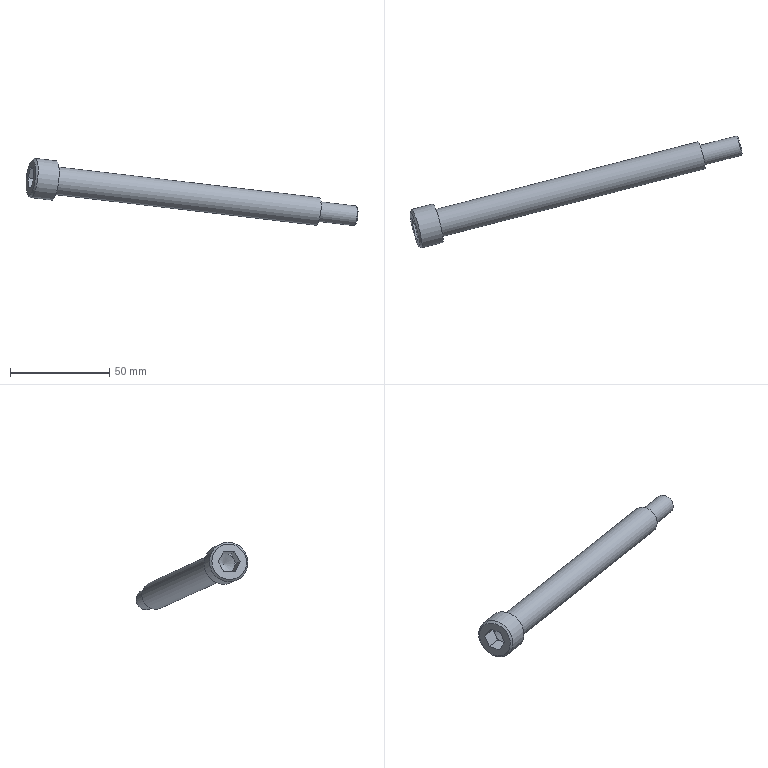Part | STEP file | 车灯-后视镜_id486_x_t | 1 solid | 22 faces | box 167.24 x 56.347 x 33.937 mm | volume 25779 mm3 | plane 16 | cylinder 3 | cone 3 | commonest cylinder face diameters 10 x1 14 x1 20 x1
STEP:
#1=CARTESIAN_POINT('',(-226.246,11.16,106.949));
#2=VERTEX_POINT('',#1);
#3=CARTESIAN_POINT('',(-227.054,15.423,109.433));
#4=VERTEX_POINT('',#3);
#5=CARTESIAN_POINT('',(-227.601,15.282,104.465));
#6=DIRECTION('',(-0.9621,-0.2482,0.113));
#7=DIRECTION('',(0.2498,-0.9683,0.));
#8=AXIS2_PLACEMENT_3D('',#5,#6,#7);
#9=CIRCLE('',#8,5.);
#10=EDGE_CURVE('',#2,#4,#9,.T.);
#11=ORIENTED_EDGE('',*,*,#10,.F.);
#12=CARTESIAN_POINT('',(-226.333,12.628,109.433));
#13=VERTEX_POINT('',#12);
#14=CARTESIAN_POINT('',(-226.159,9.691,104.465));
#15=DIRECTION('',(-0.03016,0.5086,0.8605));
#16=VECTOR('',#15,1.);
#17=LINE('',#14,#16);
#18=EDGE_CURVE('',#2,#13,#17,.T.);
#19=ORIENTED_EDGE('',*,*,#18,.T.);
#20=CARTESIAN_POINT('',(-226.333,12.628,109.433));
#21=DIRECTION('',(-0.2498,0.9683,0.));
#22=VECTOR('',#21,1.);
#23=LINE('',#20,#22);
#24=EDGE_CURVE('',#13,#4,#23,.T.);
#25=ORIENTED_EDGE('',*,*,#24,.T.);
#26=EDGE_LOOP('',(#11,#19,#25));
#27=FACE_OUTER_BOUND('',#26,.T.);
#28=CARTESIAN_POINT('',(-229.217,23.809,109.433));
#29=DIRECTION('',(-0.9621,-0.2482,0.113));
#30=DIRECTION('',(0.2498,-0.9683,0.));
#31=AXIS2_PLACEMENT_3D('',#28,#29,#30);
#32=PLANE('',#31);
#33=ADVANCED_FACE('',(#27),#32,.T.);
#34=CARTESIAN_POINT('',(-228.409,19.545,106.949));
#35=VERTEX_POINT('',#34);
#36=CARTESIAN_POINT('',(-227.601,15.282,104.465));
#37=DIRECTION('',(-0.9621,-0.2482,0.113));
#38=DIRECTION('',(0.2498,-0.9683,0.));
#39=AXIS2_PLACEMENT_3D('',#36,#37,#38);
#40=CIRCLE('',#39,5.);
#41=EDGE_CURVE('',#4,#35,#40,.T.);
#42=ORIENTED_EDGE('',*,*,#41,.F.);
#43=CARTESIAN_POINT('',(-227.775,18.218,109.433));
#44=VERTEX_POINT('',#43);
#45=CARTESIAN_POINT('',(-226.333,12.628,109.433));
#46=DIRECTION('',(-0.2498,0.9683,0.));
#47=VECTOR('',#46,1.);
#48=LINE('',#45,#47);
#49=EDGE_CURVE('',#4,#44,#48,.T.);
#50=ORIENTED_EDGE('',*,*,#49,.T.);
#51=CARTESIAN_POINT('',(-227.775,18.218,109.433));
#52=DIRECTION('',(-0.2196,0.4597,-0.8605));
#53=VECTOR('',#52,1.);
#54=LINE('',#51,#53);
#55=EDGE_CURVE('',#44,#35,#54,.T.);
#56=ORIENTED_EDGE('',*,*,#55,.T.);
#57=EDGE_LOOP('',(#42,#50,#56));
#58=FACE_OUTER_BOUND('',#57,.T.);
#59=CARTESIAN_POINT('',(-229.217,23.809,109.433));
#60=DIRECTION('',(-0.9621,-0.2482,0.113));
#61=DIRECTION('',(0.2498,-0.9683,0.));
#62=AXIS2_PLACEMENT_3D('',#59,#60,#61);
#63=PLANE('',#62);
#64=ADVANCED_FACE('',(#58),#63,.T.);
#65=CARTESIAN_POINT('',(-228.956,19.404,101.981));
#66=VERTEX_POINT('',#65);
#67=CARTESIAN_POINT('',(-227.601,15.282,104.465));
#68=DIRECTION('',(-0.9621,-0.2482,0.113));
#69=DIRECTION('',(0.2498,-0.9683,0.));
#70=AXIS2_PLACEMENT_3D('',#67,#68,#69);
#71=CIRCLE('',#70,5.);
#72=EDGE_CURVE('',#35,#66,#71,.T.);
#73=ORIENTED_EDGE('',*,*,#72,.F.);
#74=CARTESIAN_POINT('',(-229.043,20.872,104.465));
#75=VERTEX_POINT('',#74);
#76=CARTESIAN_POINT('',(-227.775,18.218,109.433));
#77=DIRECTION('',(-0.2196,0.4597,-0.8605));
#78=VECTOR('',#77,1.);
#79=LINE('',#76,#78);
#80=EDGE_CURVE('',#35,#75,#79,.T.);
#81=ORIENTED_EDGE('',*,*,#80,.T.);
#82=CARTESIAN_POINT('',(-229.043,20.872,104.465));
#83=DIRECTION('',(0.03016,-0.5086,-0.8605));
#84=VECTOR('',#83,1.);
#85=LINE('',#82,#84);
#86=EDGE_CURVE('',#75,#66,#85,.T.);
#87=ORIENTED_EDGE('',*,*,#86,.T.);
#88=EDGE_LOOP('',(#73,#81,#87));
#89=FACE_OUTER_BOUND('',#88,.T.);
#90=CARTESIAN_POINT('',(-229.217,23.809,109.433));
#91=DIRECTION('',(-0.9621,-0.2482,0.113));
#92=DIRECTION('',(0.2498,-0.9683,0.));
#93=AXIS2_PLACEMENT_3D('',#90,#91,#92);
#94=PLANE('',#93);
#95=ADVANCED_FACE('',(#89),#94,.T.);
#96=CARTESIAN_POINT('',(-228.148,15.141,99.497));
#97=VERTEX_POINT('',#96);
#98=CARTESIAN_POINT('',(-227.601,15.282,104.465));
#99=DIRECTION('',(-0.9621,-0.2482,0.113));
#100=DIRECTION('',(-0.2498,0.9683,0.));
#101=AXIS2_PLACEMENT_3D('',#98,#99,#100);
#102=CIRCLE('',#101,5.);
#103=EDGE_CURVE('',#66,#97,#102,.T.);
#104=ORIENTED_EDGE('',*,*,#103,.F.);
#105=CARTESIAN_POINT('',(-228.869,17.936,99.497));
#106=VERTEX_POINT('',#105);
#107=CARTESIAN_POINT('',(-229.043,20.872,104.465));
#108=DIRECTION('',(0.03016,-0.5086,-0.8605));
#109=VECTOR('',#108,1.);
#110=LINE('',#107,#109);
#111=EDGE_CURVE('',#66,#106,#110,.T.);
#112=ORIENTED_EDGE('',*,*,#111,.T.);
#113=CARTESIAN_POINT('',(-228.869,17.936,99.497));
#114=DIRECTION('',(0.2498,-0.9683,0.));
#115=VECTOR('',#114,1.);
#116=LINE('',#113,#115);
#117=EDGE_CURVE('',#106,#97,#116,.T.);
#118=ORIENTED_EDGE('',*,*,#117,.T.);
#119=EDGE_LOOP('',(#104,#112,#118));
#120=FACE_OUTER_BOUND('',#119,.T.);
#121=CARTESIAN_POINT('',(-229.217,23.809,109.433));
#122=DIRECTION('',(-0.9621,-0.2482,0.113));
#123=DIRECTION('',(0.2498,-0.9683,0.));
#124=AXIS2_PLACEMENT_3D('',#121,#122,#123);
#125=PLANE('',#124);
#126=ADVANCED_FACE('',(#120),#125,.T.);
#127=CARTESIAN_POINT('',(-226.793,11.018,101.981));
#128=VERTEX_POINT('',#127);
#129=CARTESIAN_POINT('',(-227.601,15.282,104.465));
#130=DIRECTION('',(-0.9621,-0.2482,0.113));
#131=DIRECTION('',(0.2498,-0.9683,0.));
#132=AXIS2_PLACEMENT_3D('',#129,#130,#131);
#133=CIRCLE('',#132,5.);
#134=EDGE_CURVE('',#97,#128,#133,.T.);
#135=ORIENTED_EDGE('',*,*,#134,.F.);
#136=CARTESIAN_POINT('',(-227.427,12.346,99.497));
#137=VERTEX_POINT('',#136);
#138=CARTESIAN_POINT('',(-228.869,17.936,99.497));
#139=DIRECTION('',(0.2498,-0.9683,0.));
#140=VECTOR('',#139,1.);
#141=LINE('',#138,#140);
#142=EDGE_CURVE('',#97,#137,#141,.T.);
#143=ORIENTED_EDGE('',*,*,#142,.T.);
#144=CARTESIAN_POINT('',(-227.427,12.346,99.497));
#145=DIRECTION('',(0.2196,-0.4597,0.8605));
#146=VECTOR('',#145,1.);
#147=LINE('',#144,#146);
#148=EDGE_CURVE('',#137,#128,#147,.T.);
#149=ORIENTED_EDGE('',*,*,#148,.T.);
#150=EDGE_LOOP('',(#135,#143,#149));
#151=FACE_OUTER_BOUND('',#150,.T.);
#152=CARTESIAN_POINT('',(-229.217,23.809,109.433));
#153=DIRECTION('',(-0.9621,-0.2482,0.113));
#154=DIRECTION('',(0.2498,-0.9683,0.));
#155=AXIS2_PLACEMENT_3D('',#152,#153,#154);
#156=PLANE('',#155);
#157=ADVANCED_FACE('',(#151),#156,.T.);
#158=CARTESIAN_POINT('',(-233.05,4.582,105.369));
#159=VERTEX_POINT('',#158);
#160=CARTESIAN_POINT('',(-235.298,13.297,105.369));
#161=DIRECTION('',(-0.9621,-0.2482,0.113));
#162=DIRECTION('',(0.2498,-0.9683,0.));
#163=AXIS2_PLACEMENT_3D('',#160,#161,#162);
#164=CIRCLE('',#163,9.);
#165=EDGE_CURVE('',#159,#159,#164,.T.);
#166=ORIENTED_EDGE('',*,*,#165,.T.);
#167=EDGE_LOOP('',(#166));
#168=FACE_BOUND('',#167,.T.);
#169=CARTESIAN_POINT('',(-234.03,10.642,110.337));
#170=VERTEX_POINT('',#169);
#171=CARTESIAN_POINT('',(-235.472,16.233,110.337));
#172=VERTEX_POINT('',#171);
#173=CARTESIAN_POINT('',(-234.03,10.642,110.337));
#174=DIRECTION('',(-0.2498,0.9683,0.));
#175=VECTOR('',#174,1.);
#176=LINE('',#173,#175);
#177=EDGE_CURVE('',#170,#172,#176,.T.);
#178=ORIENTED_EDGE('',*,*,#177,.F.);
#179=CARTESIAN_POINT('',(-233.856,7.706,105.369));
#180=VERTEX_POINT('',#179);
#181=CARTESIAN_POINT('',(-233.856,7.706,105.369));
#182=DIRECTION('',(-0.03016,0.5086,0.8605));
#183=VECTOR('',#182,1.);
#184=LINE('',#181,#183);
#185=EDGE_CURVE('',#180,#170,#184,.T.);
#186=ORIENTED_EDGE('',*,*,#185,.F.);
#187=CARTESIAN_POINT('',(-235.124,10.36,100.401));
#188=VERTEX_POINT('',#187);
#189=CARTESIAN_POINT('',(-235.124,10.36,100.401));
#190=DIRECTION('',(0.2196,-0.4597,0.8605));
#191=VECTOR('',#190,1.);
#192=LINE('',#189,#191);
#193=EDGE_CURVE('',#188,#180,#192,.T.);
#194=ORIENTED_EDGE('',*,*,#193,.F.);
#195=CARTESIAN_POINT('',(-236.566,15.951,100.401));
#196=VERTEX_POINT('',#195);
#197=CARTESIAN_POINT('',(-236.566,15.951,100.401));
#198=DIRECTION('',(0.2498,-0.9683,0.));
#199=VECTOR('',#198,1.);
#200=LINE('',#197,#199);
#201=EDGE_CURVE('',#196,#188,#200,.T.);
#202=ORIENTED_EDGE('',*,*,#201,.F.);
#203=CARTESIAN_POINT('',(-236.74,18.887,105.369));
#204=VERTEX_POINT('',#203);
#205=CARTESIAN_POINT('',(-236.74,18.887,105.369));
#206=DIRECTION('',(0.03016,-0.5086,-0.8605));
#207=VECTOR('',#206,1.);
#208=LINE('',#205,#207);
#209=EDGE_CURVE('',#204,#196,#208,.T.);
#210=ORIENTED_EDGE('',*,*,#209,.F.);
#211=CARTESIAN_POINT('',(-235.472,16.233,110.337));
#212=DIRECTION('',(-0.2196,0.4597,-0.8605));
#213=VECTOR('',#212,1.);
#214=LINE('',#211,#213);
#215=EDGE_CURVE('',#172,#204,#214,.T.);
#216=ORIENTED_EDGE('',*,*,#215,.F.);
#217=EDGE_LOOP('',(#178,#186,#194,#202,#210,#216));
#218=FACE_BOUND('',#217,.T.);
#219=CARTESIAN_POINT('',(-235.298,13.297,105.369));
#220=DIRECTION('',(-0.9621,-0.2482,0.113));
#221=DIRECTION('',(0.2498,-0.9683,0.));
#222=AXIS2_PLACEMENT_3D('',#219,#220,#221);
#223=PLANE('',#222);
#224=ADVANCED_FACE('',(#168,#218),#223,.T.);
#225=CARTESIAN_POINT('',(-225.501,23.053,104.013));
#226=VERTEX_POINT('',#225);
#227=CARTESIAN_POINT('',(-223.753,16.275,104.013));
#228=DIRECTION('',(0.9621,0.2482,-0.113));
#229=DIRECTION('',(-0.2498,0.9683,0.));
#230=AXIS2_PLACEMENT_3D('',#227,#228,#229);
#231=CIRCLE('',#230,7.);
#232=EDGE_CURVE('',#226,#226,#231,.T.);
#233=ORIENTED_EDGE('',*,*,#232,.F.);
#234=EDGE_LOOP('',(#233));
#235=FACE_BOUND('',#234,.T.);
#236=CARTESIAN_POINT('',(-226.25,25.958,104.013));
#237=VERTEX_POINT('',#236);
#238=CARTESIAN_POINT('',(-223.753,16.275,104.013));
#239=DIRECTION('',(-0.9621,-0.2482,0.113));
#240=DIRECTION('',(-0.2498,0.9683,0.));
#241=AXIS2_PLACEMENT_3D('',#238,#239,#240);
#242=CIRCLE('',#241,10.);
#243=EDGE_CURVE('',#237,#237,#242,.T.);
#244=ORIENTED_EDGE('',*,*,#243,.F.);
#245=EDGE_LOOP('',(#244));
#246=FACE_BOUND('',#245,.T.);
#247=CARTESIAN_POINT('',(-223.753,16.275,104.013));
#248=DIRECTION('',(0.9621,0.2482,-0.113));
#249=DIRECTION('',(-0.2498,0.9683,0.));
#250=AXIS2_PLACEMENT_3D('',#247,#248,#249);
#251=PLANE('',#250);
#252=ADVANCED_FACE('',(#235,#246),#251,.T.);
#253=CARTESIAN_POINT('',(-231.838,3.862,105.256));
#254=VERTEX_POINT('',#253);
#255=CARTESIAN_POINT('',(-234.336,13.545,105.256));
#256=DIRECTION('',(0.9621,0.2482,-0.113));
#257=DIRECTION('',(0.2498,-0.9683,0.));
#258=AXIS2_PLACEMENT_3D('',#255,#256,#257);
#259=CIRCLE('',#258,10.);
#260=EDGE_CURVE('',#254,#254,#259,.T.);
#261=ORIENTED_EDGE('',*,*,#260,.T.);
#262=EDGE_LOOP('',(#261));
#263=FACE_BOUND('',#262,.T.);
#264=ORIENTED_EDGE('',*,*,#243,.T.);
#265=EDGE_LOOP('',(#264));
#266=FACE_BOUND('',#265,.T.);
#267=CARTESIAN_POINT('',(-228.563,15.034,104.578));
#268=DIRECTION('',(-0.9621,-0.2482,0.113));
#269=DIRECTION('',(0.2498,-0.9683,0.));
#270=AXIS2_PLACEMENT_3D('',#267,#268,#269);
#271=CYLINDRICAL_SURFACE('',#270,10.);
#272=ADVANCED_FACE('',(#263,#266),#271,.T.);
#273=CARTESIAN_POINT('',(-92.23,55.363,88.426));
#274=VERTEX_POINT('',#273);
#275=CARTESIAN_POINT('',(-90.981,50.522,88.426));
#276=DIRECTION('',(0.9621,0.2482,-0.113));
#277=DIRECTION('',(-0.2498,0.9683,0.));
#278=AXIS2_PLACEMENT_3D('',#275,#276,#277);
#279=CIRCLE('',#278,5.);
#280=EDGE_CURVE('',#274,#274,#279,.T.);
#281=ORIENTED_EDGE('',*,*,#280,.F.);
#282=EDGE_LOOP('',(#281));
#283=FACE_BOUND('',#282,.T.);
#284=CARTESIAN_POINT('',(-92.73,57.3,88.426));
#285=VERTEX_POINT('',#284);
#286=CARTESIAN_POINT('',(-90.981,50.522,88.426));
#287=DIRECTION('',(-0.9621,-0.2482,0.113));
#288=DIRECTION('',(-0.2498,0.9683,0.));
#289=AXIS2_PLACEMENT_3D('',#286,#287,#288);
#290=CIRCLE('',#289,7.);
#291=EDGE_CURVE('',#285,#285,#290,.T.);
#292=ORIENTED_EDGE('',*,*,#291,.F.);
#293=EDGE_LOOP('',(#292));
#294=FACE_BOUND('',#293,.T.);
#295=CARTESIAN_POINT('',(-90.981,50.522,88.426));
#296=DIRECTION('',(0.9621,0.2482,-0.113));
#297=DIRECTION('',(-0.2498,0.9683,0.));
#298=AXIS2_PLACEMENT_3D('',#295,#296,#297);
#299=PLANE('',#298);
#300=ADVANCED_FACE('',(#283,#294),#299,.T.);
#301=ORIENTED_EDGE('',*,*,#232,.T.);
#302=EDGE_LOOP('',(#301));
#303=FACE_BOUND('',#302,.T.);
#304=ORIENTED_EDGE('',*,*,#291,.T.);
#305=EDGE_LOOP('',(#304));
#306=FACE_BOUND('',#305,.T.);
#307=CARTESIAN_POINT('',(-95.792,49.281,88.99));
#308=DIRECTION('',(-0.9621,-0.2482,0.113));
#309=DIRECTION('',(0.2498,-0.9683,0.));
#310=AXIS2_PLACEMENT_3D('',#307,#308,#309);
#311=CYLINDRICAL_SURFACE('',#310,7.);
#312=ADVANCED_FACE('',(#303,#306),#311,.T.);
#313=CARTESIAN_POINT('',(-72.863,59.843,86.167));
#314=VERTEX_POINT('',#313);
#315=CARTESIAN_POINT('',(-71.739,55.485,86.167));
#316=DIRECTION('',(0.9621,0.2482,-0.113));
#317=DIRECTION('',(-0.2498,0.9683,0.));
#318=AXIS2_PLACEMENT_3D('',#315,#316,#317);
#319=CIRCLE('',#318,4.5);
#320=EDGE_CURVE('',#314,#314,#319,.T.);
#321=ORIENTED_EDGE('',*,*,#320,.T.);
#322=EDGE_LOOP('',(#321));
#323=FACE_OUTER_BOUND('',#322,.T.);
#324=CARTESIAN_POINT('',(-71.739,55.485,86.167));
#325=DIRECTION('',(0.9621,0.2482,-0.113));
#326=DIRECTION('',(-0.2498,0.9683,0.));
#327=AXIS2_PLACEMENT_3D('',#324,#325,#326);
#328=PLANE('',#327);
#329=ADVANCED_FACE('',(#323),#328,.T.);
#330=CARTESIAN_POINT('',(-73.469,60.203,86.223));
#331=VERTEX_POINT('',#330);
#332=CARTESIAN_POINT('',(-72.22,55.361,86.223));
#333=DIRECTION('',(-0.9621,-0.2482,0.113));
#334=DIRECTION('',(-0.2498,0.9683,0.));
#335=AXIS2_PLACEMENT_3D('',#332,#333,#334);
#336=CIRCLE('',#335,5.);
#337=EDGE_CURVE('',#331,#331,#336,.T.);
#338=ORIENTED_EDGE('',*,*,#337,.T.);
#339=EDGE_LOOP('',(#338));
#340=FACE_BOUND('',#339,.T.);
#341=ORIENTED_EDGE('',*,*,#280,.T.);
#342=EDGE_LOOP('',(#341));
#343=FACE_BOUND('',#342,.T.);
#344=CARTESIAN_POINT('',(-90.981,50.522,88.426));
#345=DIRECTION('',(0.9621,0.2482,-0.113));
#346=DIRECTION('',(-0.2498,0.9683,0.));
#347=AXIS2_PLACEMENT_3D('',#344,#345,#346);
#348=CYLINDRICAL_SURFACE('',#347,5.);
#349=ADVANCED_FACE('',(#340,#343),#348,.T.);
#350=ORIENTED_EDGE('',*,*,#320,.F.);
#351=EDGE_LOOP('',(#350));
#352=FACE_BOUND('',#351,.T.);
#353=ORIENTED_EDGE('',*,*,#337,.F.);
#354=EDGE_LOOP('',(#353));
#355=FACE_BOUND('',#354,.T.);
#356=CARTESIAN_POINT('',(-72.22,55.361,86.223));
#357=DIRECTION('',(-0.9621,-0.2482,0.113));
#358=DIRECTION('',(0.2498,-0.9683,0.));
#359=AXIS2_PLACEMENT_3D('',#356,#357,#358);
#360=CONICAL_SURFACE('',#359,5.,45.);
#361=ADVANCED_FACE('',(#352,#355),#360,.T.);
#362=ORIENTED_EDGE('',*,*,#177,.T.);
#363=CARTESIAN_POINT('',(-227.775,18.218,109.433));
#364=DIRECTION('',(-0.9621,-0.2482,0.113));
#365=VECTOR('',#364,1.);
#366=LINE('',#363,#365);
#367=EDGE_CURVE('',#44,#172,#366,.T.);
#368=ORIENTED_EDGE('',*,*,#367,.F.);
#369=ORIENTED_EDGE('',*,*,#49,.F.);
#370=ORIENTED_EDGE('',*,*,#24,.F.);
#371=CARTESIAN_POINT('',(-226.333,12.628,109.433));
#372=DIRECTION('',(-0.9621,-0.2482,0.113));
#373=VECTOR('',#372,1.);
#374=LINE('',#371,#373);
#375=EDGE_CURVE('',#13,#170,#374,.T.);
#376=ORIENTED_EDGE('',*,*,#375,.T.);
#377=EDGE_LOOP('',(#362,#368,#369,#370,#376));
#378=FACE_OUTER_BOUND('',#377,.T.);
#379=CARTESIAN_POINT('',(-226.333,12.628,109.433));
#380=DIRECTION('',(0.1094,0.02821,0.9936));
#381=DIRECTION('',(0.994,0.,-0.1094));
#382=AXIS2_PLACEMENT_3D('',#379,#380,#381);
#383=PLANE('',#382);
#384=ADVANCED_FACE('',(#378),#383,.F.);
#385=ORIENTED_EDGE('',*,*,#215,.T.);
#386=CARTESIAN_POINT('',(-229.043,20.872,104.465));
#387=DIRECTION('',(-0.9621,-0.2482,0.113));
#388=VECTOR('',#387,1.);
#389=LINE('',#386,#388);
#390=EDGE_CURVE('',#75,#204,#389,.T.);
#391=ORIENTED_EDGE('',*,*,#390,.F.);
#392=ORIENTED_EDGE('',*,*,#80,.F.);
#393=ORIENTED_EDGE('',*,*,#55,.F.);
#394=ORIENTED_EDGE('',*,*,#367,.T.);
#395=EDGE_LOOP('',(#385,#391,#392,#393,#394));
#396=FACE_OUTER_BOUND('',#395,.T.);
#397=CARTESIAN_POINT('',(-227.775,18.218,109.433));
#398=DIRECTION('',(-0.1616,0.8527,0.4968));
#399=DIRECTION('',(0.,-0.5034,0.864));
#400=AXIS2_PLACEMENT_3D('',#397,#398,#399);
#401=PLANE('',#400);
#402=ADVANCED_FACE('',(#396),#401,.F.);
#403=ORIENTED_EDGE('',*,*,#209,.T.);
#404=CARTESIAN_POINT('',(-228.869,17.936,99.497));
#405=DIRECTION('',(-0.9621,-0.2482,0.113));
#406=VECTOR('',#405,1.);
#407=LINE('',#404,#406);
#408=EDGE_CURVE('',#106,#196,#407,.T.);
#409=ORIENTED_EDGE('',*,*,#408,.F.);
#410=ORIENTED_EDGE('',*,*,#111,.F.);
#411=ORIENTED_EDGE('',*,*,#86,.F.);
#412=ORIENTED_EDGE('',*,*,#390,.T.);
#413=EDGE_LOOP('',(#403,#409,#410,#411,#412));
#414=FACE_OUTER_BOUND('',#413,.T.);
#415=CARTESIAN_POINT('',(-229.043,20.872,104.465));
#416=DIRECTION('',(-0.271,0.8245,-0.4968));
#417=DIRECTION('',(0.,0.5161,0.8565));
#418=AXIS2_PLACEMENT_3D('',#415,#416,#417);
#419=PLANE('',#418);
#420=ADVANCED_FACE('',(#414),#419,.F.);
#421=ORIENTED_EDGE('',*,*,#201,.T.);
#422=CARTESIAN_POINT('',(-227.427,12.346,99.497));
#423=DIRECTION('',(-0.9621,-0.2482,0.113));
#424=VECTOR('',#423,1.);
#425=LINE('',#422,#424);
#426=EDGE_CURVE('',#137,#188,#425,.T.);
#427=ORIENTED_EDGE('',*,*,#426,.F.);
#428=ORIENTED_EDGE('',*,*,#142,.F.);
#429=ORIENTED_EDGE('',*,*,#117,.F.);
#430=ORIENTED_EDGE('',*,*,#408,.T.);
#431=EDGE_LOOP('',(#421,#427,#428,#429,#430));
#432=FACE_OUTER_BOUND('',#431,.T.);
#433=CARTESIAN_POINT('',(-228.869,17.936,99.497));
#434=DIRECTION('',(-0.1094,-0.02821,-0.9936));
#435=DIRECTION('',(-0.994,0.,0.1094));
#436=AXIS2_PLACEMENT_3D('',#433,#434,#435);
#437=PLANE('',#436);
#438=ADVANCED_FACE('',(#432),#437,.F.);
#439=ORIENTED_EDGE('',*,*,#193,.T.);
#440=CARTESIAN_POINT('',(-226.159,9.691,104.465));
#441=VERTEX_POINT('',#440);
#442=CARTESIAN_POINT('',(-226.159,9.691,104.465));
#443=DIRECTION('',(-0.9621,-0.2482,0.113));
#444=VECTOR('',#443,1.);
#445=LINE('',#442,#444);
#446=EDGE_CURVE('',#441,#180,#445,.T.);
#447=ORIENTED_EDGE('',*,*,#446,.F.);
#448=CARTESIAN_POINT('',(-227.427,12.346,99.497));
#449=DIRECTION('',(0.2196,-0.4597,0.8605));
#450=VECTOR('',#449,1.);
#451=LINE('',#448,#450);
#452=EDGE_CURVE('',#128,#441,#451,.T.);
#453=ORIENTED_EDGE('',*,*,#452,.F.);
#454=ORIENTED_EDGE('',*,*,#148,.F.);
#455=ORIENTED_EDGE('',*,*,#426,.T.);
#456=EDGE_LOOP('',(#439,#447,#453,#454,#455));
#457=FACE_OUTER_BOUND('',#456,.T.);
#458=CARTESIAN_POINT('',(-227.427,12.346,99.497));
#459=DIRECTION('',(0.1616,-0.8527,-0.4968));
#460=DIRECTION('',(0.,0.5034,-0.864));
#461=AXIS2_PLACEMENT_3D('',#458,#459,#460);
#462=PLANE('',#461);
#463=ADVANCED_FACE('',(#457),#462,.F.);
#464=ORIENTED_EDGE('',*,*,#185,.T.);
#465=ORIENTED_EDGE('',*,*,#375,.F.);
#466=ORIENTED_EDGE('',*,*,#18,.F.);
#467=CARTESIAN_POINT('',(-226.159,9.691,104.465));
#468=DIRECTION('',(-0.03016,0.5086,0.8605));
#469=VECTOR('',#468,1.);
#470=LINE('',#467,#469);
#471=EDGE_CURVE('',#441,#2,#470,.T.);
#472=ORIENTED_EDGE('',*,*,#471,.F.);
#473=ORIENTED_EDGE('',*,*,#446,.T.);
#474=EDGE_LOOP('',(#464,#465,#466,#472,#473));
#475=FACE_OUTER_BOUND('',#474,.T.);
#476=CARTESIAN_POINT('',(-226.159,9.691,104.465));
#477=DIRECTION('',(0.271,-0.8245,0.4968));
#478=DIRECTION('',(0.,-0.5161,-0.8565));
#479=AXIS2_PLACEMENT_3D('',#476,#477,#478);
#480=PLANE('',#479);
#481=ADVANCED_FACE('',(#475),#480,.F.);
#482=CARTESIAN_POINT('',(-227.601,15.282,104.465));
#483=DIRECTION('',(-0.9621,-0.2482,0.113));
#484=DIRECTION('',(0.2498,-0.9683,0.));
#485=AXIS2_PLACEMENT_3D('',#482,#483,#484);
#486=CIRCLE('',#485,5.);
#487=EDGE_CURVE('',#128,#2,#486,.T.);
#488=ORIENTED_EDGE('',*,*,#487,.F.);
#489=ORIENTED_EDGE('',*,*,#452,.T.);
#490=ORIENTED_EDGE('',*,*,#471,.T.);
#491=EDGE_LOOP('',(#488,#489,#490));
#492=FACE_OUTER_BOUND('',#491,.T.);
#493=CARTESIAN_POINT('',(-229.217,23.809,109.433));
#494=DIRECTION('',(-0.9621,-0.2482,0.113));
#495=DIRECTION('',(0.2498,-0.9683,0.));
#496=AXIS2_PLACEMENT_3D('',#493,#494,#495);
#497=PLANE('',#496);
#498=ADVANCED_FACE('',(#492),#497,.T.);
#499=CARTESIAN_POINT('',(-224.715,16.026,104.126));
#500=VERTEX_POINT('',#499);
#501=VERTEX_LOOP('',#500);
#502=FACE_BOUND('',#501,.T.);
#503=ORIENTED_EDGE('',*,*,#103,.T.);
#504=ORIENTED_EDGE('',*,*,#134,.T.);
#505=ORIENTED_EDGE('',*,*,#487,.T.);
#506=ORIENTED_EDGE('',*,*,#10,.T.);
#507=ORIENTED_EDGE('',*,*,#41,.T.);
#508=ORIENTED_EDGE('',*,*,#72,.T.);
#509=EDGE_LOOP('',(#503,#504,#505,#506,#507,#508));
#510=FACE_BOUND('',#509,.T.);
#511=CARTESIAN_POINT('',(-227.601,15.282,104.465));
#512=DIRECTION('',(-0.9621,-0.2482,0.113));
#513=DIRECTION('',(0.2498,-0.9683,0.));
#514=AXIS2_PLACEMENT_3D('',#511,#512,#513);
#515=CONICAL_SURFACE('',#514,5.,59.036);
#516=ADVANCED_FACE('',(#502,#510),#515,.F.);
#517=ORIENTED_EDGE('',*,*,#165,.F.);
#518=EDGE_LOOP('',(#517));
#519=FACE_BOUND('',#518,.T.);
#520=ORIENTED_EDGE('',*,*,#260,.F.);
#521=EDGE_LOOP('',(#520));
#522=FACE_BOUND('',#521,.T.);
#523=CARTESIAN_POINT('',(-234.336,13.545,105.256));
#524=DIRECTION('',(0.9621,0.2482,-0.113));
#525=DIRECTION('',(-0.2498,0.9683,0.));
#526=AXIS2_PLACEMENT_3D('',#523,#524,#525);
#527=CONICAL_SURFACE('',#526,10.,45.);
#528=ADVANCED_FACE('',(#519,#522),#527,.T.);
#529=CLOSED_SHELL('',(#33,#64,#95,#126,#157,#224,#252,#272,#300,#312,#329,#349,#361,#384,#402,#420,#438,#463,#481,#498,#516,#528));
#530=MANIFOLD_SOLID_BREP('',#529);
#531=(LENGTH_UNIT()NAMED_UNIT(*)SI_UNIT(.MILLI.,.METRE.));
#532=UNCERTAINTY_MEASURE_WITH_UNIT(LENGTH_MEASURE(0.00002),#531,'','');
#533=(NAMED_UNIT(*)PLANE_ANGLE_UNIT()SI_UNIT($,.RADIAN.));
#534=PLANE_ANGLE_MEASURE_WITH_UNIT(PLANE_ANGLE_MEASURE(0.01745),#533);
#535=DIMENSIONAL_EXPONENTS(0.,0.,0.,0.,0.,0.,0.);
#536=(CONVERSION_BASED_UNIT('DEGREE',#534)NAMED_UNIT(#535)PLANE_ANGLE_UNIT());
#537=(NAMED_UNIT(*)SI_UNIT($,.STERADIAN.)SOLID_ANGLE_UNIT());
#538=(GEOMETRIC_REPRESENTATION_CONTEXT(3)GLOBAL_UNCERTAINTY_ASSIGNED_CONTEXT((#532))GLOBAL_UNIT_ASSIGNED_CONTEXT((#531,#536,#537))REPRESENTATION_CONTEXT('',''));
#539=ADVANCED_BREP_SHAPE_REPRESENTATION('',(#530),#538);